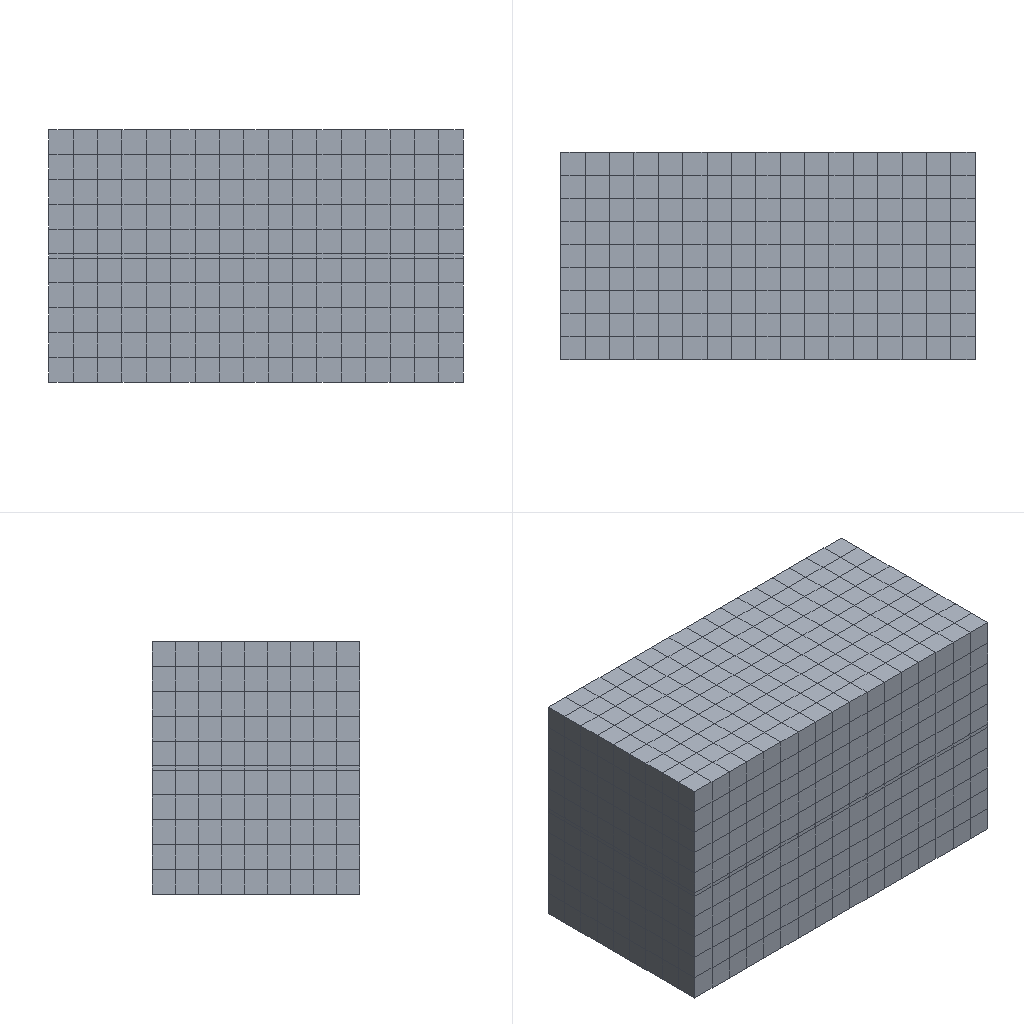Simulation study | ansys workbench
Ansys APDL input file, long lists of numbers shortened:
/batch
/config,noeldb,1     ! force off writing results to database
*get,_wallstrt,active,,time,wall
! ANSYS input file written by Workbench version 2022 R2
! File used for geometry attach:
/title,wbnew--___ (A5)
! ****** Begin Custom Load Command Snippet ******
/COM, ACT Extensions:
/COM,     LSDYNA, 2022.2
/COM,/COM,     ANSYSMotion, 2022.2
/COM,
! ****** End   Custom Load Command Snippet ******
*DIM,_wb_ProjectScratch_dir,string,248
_wb_ProjectScratch_dir(1) = ''
*DIM,_wb_SolverFiles_dir,string,248
_wb_SolverFiles_dir(1) = ''
*DIM,_wb_userfiles_dir,string,248
_wb_userfiles_dir(1) = ''
/com,--- Data in consistent NMM units. See Solving Units in the help system for more information.
/units,MPA
/nopr
/wb,file,start              !  signify a WB generated input file
/prep7
! Turn off shape checking because checks already performed inside WB mesher.
! See help system for more information.
SHPP,OFF,,NOWARN
/nolist
etcon,set             ! allow ANSYS to choose best KEYOP's for 180x elements, resets any applicable keyopt to MAPDL defaults
/com,*********** Nodes for the whole assembly ***********
nblock,3,,10062
(1i9,3e20.9e3)
     7945     4.411764706E+00     1.944444444E+00     3.000000000E+00
! (9147 more lines like these left out)
-1
/wb,elem,start            !  set before creation of elements
/com,*********** Elements for Body 1 "__" ***********
et,1,279
eblock,19,solid,,765
(19i9)
        1        1        1        1        0        0        0        0       20        0        1        1     1001      862      824      640     1080      861      853
! (1529 more lines like these left out)
-1
/com,*********** Elements for Body 2 "__" ***********
et,2,279
eblock,19,solid,,765
(19i9)
        2        2        2        2        0        0        0        0       20        0      766     3973     4793     4874     5041     4612     4872     4873     5045
! (1529 more lines like these left out)
-1
/com,*********** Elements for Body 3 "__" ***********
et,3,279
eblock,19,solid,,153
(19i9)
        3        3        3        3        0        0        0        0       20        0     1531     8072     8297     8269     8268     8073     8208     8235     8236
! (305 more lines like these left out)
-1
/wb,elem,end               !  done creating elements
/com,*********** Send User Defined Coordinate System(s) ***********
csys,0
toffst,273.15,  ! Temperature offset from absolute zero
/wb,mat,start              !  starting to send materials
/com,*********** Send Materials ***********
MP,DENS,1,3.2e-09,	! tonne mm^-3
MP,ALPX,1,3.5e-06,	! C^-1
MP,KXX,1,20,	! tonne mm s^-3 C^-1
MP,C,1,750000000,	! mm^2 s^-2 C^-1
MP,EX,1,300000,	! tonne s^-2 mm^-1
MP,NUXY,1,0.27,
Temperature = 'TEMP' ! Temperature
MP,DENS,2,4.51e-09,	! tonne mm^-3
MP,CTEX,2,9e-06,	! C^-1
MP,C,2,530000000,	! mm^2 s^-2 C^-1
MP,KXX,2,19,	! tonne mm s^-3 C^-1
MP,RSVX,2,0.0017,	! ohm mm
MP,EX,2,110000,	! tonne s^-2 mm^-1
MP,NUXY,2,0.34,
MP,MURX,2,1,
MP,DENS,3,9.8e-09,	! tonne mm^-3
MP,CTEX,3,1.9e-05,	! C^-1
MP,EX,3,75000,	! tonne s^-2 mm^-1
MP,NUXY,3,0.35,
MP,KXX,3,110,	! tonne mm s^-3 C^-1
MP,C,3,420000000,	! mm^2 s^-2 C^-1
/wb,mat,end                !  done sending materials
!************************* Model Summary ********************
!__,	SI3N4,	matid,	1
!__,	钛合金,	matid,	2
!__,	AG-CU-TI,	matid,	3
!************************* End Model Summary ********************
! get the diagonal of the bounding box. Needed later for other things
*get,_xmin,node,,mnloc,x
*get,_ymin,node,,mnloc,y
*get,_zmin,node,,mnloc,z
*get,_xmax,node,,mxloc,x
*get,_ymax,node,,mxloc,y
*get,_zmax,node,,mxloc,z
_ASMDIAG=(_xmax-_xmin)*(_xmax-_xmin)+(_ymax-_ymin)*(_ymax-_ymin)+(_zmax-_zmin)*(_zmax-_zmin)
_ASMDIAG=SQRT(_ASMDIAG)
/wb,contact,start          !  starting to send contact
/com,*********** Create Contact "接触区域" ***********
/com,            Real Constant Set For Above Contact Is 5 & 4
*set,tid,5
*set,cid,4
r,tid
r,cid
et,tid,170
et,cid,174
eblock,10,,,153
(15i9)
     3174        5        5        5        0      853      640     1080      861     3119     3120     3583     3574
! (152 more lines like these left out)
-1
eblock,10,,,153
(15i9)
     3327        4        4        4        0      853      640     1080      861     3119     3120     3583     3574
! (152 more lines like these left out)
-1
eblock,10,,,153
(15i9)
     3480        4        5        4        0     8236     8073     8208     8235     8716     8715     9008     9062
! (152 more lines like these left out)
-1
eblock,10,,,153
(15i9)
     3633        5        4        5        0     8236     8073     8208     8235     8716     8715     9008     9062
! (152 more lines like these left out)
-1
keyo,cid,8,2               ! auto create asymmetric contact (from Program Controlled setting)
keyo,cid,10,0              ! adjust contact stiffness each NR iteration (from Program Controlled setting)
keyo,cid,12,5              ! bonded always
keyo,cid,18,1              ! small sliding turned on by application
keyo,cid,2,0               ! augmented Lagrange (from Program Controlled setting)
keyo,cid,4,0               ! on Gauss point (from Program Controlled setting)
keyo,cid,9,1               ! ignore initial gaps/penetration
keyo,cid,7,0               ! No Prediction
rmod,tid,3,10.      ! FKN
rmod,tid,5,0.       ! ICONT
rmod,tid,6,0.       ! PINB
rmod,tid,10,0.      ! CNOF
rmod,tid,12,0.      ! FKT
rmod,tid,36,34      ! WB DSID
rmod,cid,3,10.      ! FKN
rmod,cid,5,0.       ! ICONT
rmod,cid,6,0.       ! PINB
rmod,cid,10,0.      ! CNOF
rmod,cid,12,0.      ! FKT
rmod,cid,36,34      ! WB DSID
*set,_maxkxx,1100000.
rmod,cid,14,_maxkxx/_ASMDIAG         ! TCC, Divide by Length since Traction Based
rmod,tid,14,_maxkxx/_ASMDIAG      ! TCC, Divide by Length since Traction Based
keyo,cid,1,2     ! Pure thermal contact
/com,*********** Create Contact "接触区域 2" ***********
/com,            Real Constant Set For Above Contact Is 7 & 6
*set,tid,7
*set,cid,6
r,tid
r,cid
et,tid,170
et,cid,174
eblock,10,,,153
(15i9)
     3786        7        7        7        0     4776     4613     4748     4775     7096     7095     7388     7442
! (152 more lines like these left out)
-1
eblock,10,,,153
(15i9)
     3939        6        6        6        0     4776     4613     4748     4775     7096     7095     7388     7442
! (152 more lines like these left out)
-1
eblock,10,,,153
(15i9)
     4092        6        7        6        0     8297     8072     8268     8269     8712     8711     9113     9114
! (152 more lines like these left out)
-1
eblock,10,,,153
(15i9)
     4245        7        6        7        0     8297     8072     8268     8269     8712     8711     9113     9114
! (152 more lines like these left out)
-1
keyo,cid,8,2               ! auto create asymmetric contact (from Program Controlled setting)
keyo,cid,10,0              ! adjust contact stiffness each NR iteration (from Program Controlled setting)
keyo,cid,12,5              ! bonded always
keyo,cid,18,1              ! small sliding turned on by application
keyo,cid,2,0               ! augmented Lagrange (from Program Controlled setting)
keyo,cid,4,0               ! on Gauss point (from Program Controlled setting)
keyo,cid,9,1               ! ignore initial gaps/penetration
keyo,cid,7,0               ! No Prediction
rmod,tid,3,10.      ! FKN
rmod,tid,5,0.       ! ICONT
rmod,tid,6,0.       ! PINB
rmod,tid,10,0.      ! CNOF
rmod,tid,12,0.      ! FKT
rmod,tid,36,37      ! WB DSID
rmod,cid,3,10.      ! FKN
rmod,cid,5,0.       ! ICONT
rmod,cid,6,0.       ! PINB
rmod,cid,10,0.      ! CNOF
rmod,cid,12,0.      ! FKT
rmod,cid,36,37      ! WB DSID
*set,_maxkxx,1100000.
rmod,cid,14,_maxkxx/_ASMDIAG         ! TCC, Divide by Length since Traction Based
rmod,tid,14,_maxkxx/_ASMDIAG      ! TCC, Divide by Length since Traction Based
keyo,cid,1,2     ! Pure thermal contact
nsel,all
esel,all
/wb,contact,end            !  done creating contacts
/golist
/wb,load,start             !  starting to send loads
/com,*********** Create "热流" ***********
et,8,152
eblock,10,,,17
(15i9)
     4398        8        8        8        0     8268     8236     8235     8269     9065     9062     9063     9113
! (16 more lines like these left out)
-1
esel,s,type,,8
keyop,8,8,1      ! include heat flux
esel,all
fcum,add                   ! add nodal forces up (needed in case have loads on the same edge,vertex)
nsel,all
nsel,all
fcum                       ! reset default on fcum command since done sending WB F loads
/com,*********** Create "______" ***********
et,9,152
eblock,10,,,826
(15i9)
     4415        9        9        9        0     1080     1001      862      861     3836     3585     3582     3583
! (825 more lines like these left out)
-1
esel,s,type,,9
keyop,9,8,2.
keyop,9,13,0
*DIM,_convvari62,TABLE,8,1,1,TEMP,
! Temperature values
_convvari62(1,0,1) = 1.
_convvari62(2,0,1) = 10.
_convvari62(3,0,1) = 100.
_convvari62(4,0,1) = 200.
_convvari62(5,0,1) = 300.
_convvari62(6,0,1) = 500.
_convvari62(7,0,1) = 700.
_convvari62(8,0,1) = 1000.
! Load values
_convvari62(1,1,1) = 1.24e-003
_convvari62(2,1,1) = 2.67e-003
_convvari62(3,1,1) = 5.76e-003
_convvari62(4,1,1) = 7.25e-003
_convvari62(5,1,1) = 8.3e-003
_convvari62(6,1,1) = 9.84e-003
_convvari62(7,1,1) = 1.101e-002
_convvari62(8,1,1) = 1.24e-002
esel,all
/com,*********** Create "ToAmbient" Radiation ***********
n,9149,_ASMDIAG*0.5*1,0.,0.
nsel,s,node,,9149
cm,_SPND64,node
nsel,all
et,10,152
keyop,10,5,1        !  Extra node
keyop,10,9,1        !  Use radiation with the form factor real constant
eblock,10,,,1490
(15i9)
     5241       10       10       10        0      819      821      865      820     3503     3507     3504     3502     9149
! (1489 more lines like these left out)
-1
esel,s,type,,10
mp,emis,10,0.3
r,10,1.,5.669e-011
stef,5.669e-011
esel,all
nsel,all
/com,***************** Define Uniform Initial temperature ***************
tunif,25.
/gst,on,on
fini
*get,_numnode,node,0,count
*get,_numelem,elem,0,count
*get, _MAXELEMNUM, elem, 0, NUM, MAX
*get, _MAXNODENUM, node, 0, NUM, MAX
*get, _MAXELEMTYPE, etyp, 0, NUM, MAX
*get, _MAXREALCONST, rcon, 0, NUM, MAX
/go
/wb,load,end               !  done creating loads
/com,--- Number of total nodes = %_numnode%
/com,--- Number of contact elements = 3557
/com,--- Number of spring elements = 0
/com,--- Number of bearing elements = 0
/com,--- Number of solid elements = 1683
/com,--- Number of condensed parts = 0
/com,--- Number of total elements = %_numelem%
*get,_wallbsol,active,,time,wall
/com,****************************************************************************
/com,*************************    SOLUTION       ********************************
/com,****************************************************************************
/solu
antype,4                   ! transient analysis
kbc,1                      ! stepped BC's
!eqsl,sparse               ! using sparse solver which is default so no eqsl command needed
cntr,print,1               ! print out contact info and also make no initial contact an error
rescontrol,,none                 ! Do not keep any restart files
dmpoption,emat,no             ! Don't combine emat file for DANSYS
dmpoption,esav,no             ! Don't combine esav file for DANSYS
thopt,full
nlhist,nsol,MAX_TEMP,temp,max
nlhist,nsol,MIN_TEMP,temp,min
/com,********* Initial Time Increment Check And Fourier Modulus *********
/com, Specified Initial Time Increment: 0.01
/com, Estimated Increment Needed, le*le/alpha, Body 1: 0.0405
/com, Estimated Increment Needed, le*le/alpha, Body 2: 0.04246
/com, Estimated Increment Needed, le*le/alpha, Body 3: 0.003825
/com,****************************************************
/com,******************* SOLVE FOR LS 1 OF 5 ****************
esel,s,type,,8
nsle
sf,all,hflux,200000.
nsel,all
esel,all
esel,s,type,,9
nsle
sf,all,conv,%_convvari62%,25.
nsel,all
esel,all
d,_SPND64,temp,25.
/nopr
/gopr
autots,on
nsub,100,1000,10
time,1.
timint,on                  ! Turn on time integration effects
outres,erase
outres,all,none
outres,nsol,all
outres,rsol,all
outres,eangl,all
outres,veng,all
outres,fflux,all
outres,cont,all
/nopr
esel,s,type,,9
esel,a,type,,10
cm,_elmisc,elem
esel,all
/gopr
outres,misc,all,_elmisc
cnvtol,heat,,.001,,1.e-003    ! Program Controlled. Set MINREF equivalent of 1e-6 Watts
! *********** WB SOLVE COMMAND ***********
! check interactive state
*get,ANSINTER_,active,,int
*if,ANSINTER_,ne,0,then
/eof
*endif
solve
/com *************** Write FE CONNECTORS *********
CEWRITE,file,ce,,INTE
/com,****************************************************
/com,*************** FINISHED SOLVE FOR LS 1 *************
/com,****************************************************
/com,******************* SOLVE FOR LS 2 OF 5 ****************
/nopr
/gopr
autots,on
nsub,100,1000,10
time,2.
timint,on                  ! Turn on time integration effects
outres,erase
outres,all,none
outres,nsol,all
outres,rsol,all
outres,eangl,all
outres,veng,all
outres,fflux,all
outres,cont,all
outres,misc,all,_elmisc
cnvtol,heat,,.001,,1.e-003    ! Program Controlled. Set MINREF equivalent of 1e-6 Watts
solve
/com,****************************************************
/com,*************** FINISHED SOLVE FOR LS 2 *************
/com,****************************************************
/com,******************* SOLVE FOR LS 3 OF 5 ****************
/nopr
/gopr
autots,on
nsub,100,1000,10
time,3.
timint,on                  ! Turn on time integration effects
outres,erase
outres,all,none
outres,nsol,all
outres,rsol,all
outres,eangl,all
outres,veng,all
outres,fflux,all
outres,cont,all
outres,misc,all,_elmisc
cnvtol,heat,,.001,,1.e-003    ! Program Controlled. Set MINREF equivalent of 1e-6 Watts
solve
/com,****************************************************
/com,*************** FINISHED SOLVE FOR LS 3 *************
/com,****************************************************
/com,******************* SOLVE FOR LS 4 OF 5 ****************
/nopr
/gopr
autots,on
nsub,100,1000,10
time,4.
timint,on                  ! Turn on time integration effects
outres,erase
outres,all,none
outres,nsol,all
outres,rsol,all
outres,eangl,all
outres,veng,all
outres,fflux,all
outres,cont,all
outres,misc,all,_elmisc
cnvtol,heat,,.001,,1.e-003    ! Program Controlled. Set MINREF equivalent of 1e-6 Watts
solve
/com,****************************************************
/com,*************** FINISHED SOLVE FOR LS 4 *************
/com,****************************************************
/com,******************* SOLVE FOR LS 5 OF 5 ****************
/nopr
/gopr
autots,on
nsub,100,1000,10
time,5.
timint,on                  ! Turn on time integration effects
outres,erase
outres,all,none
outres,nsol,all
outres,rsol,all
outres,eangl,all
outres,veng,all
outres,fflux,all
outres,cont,all
outres,misc,all,_elmisc
cnvtol,heat,,.001,,1.e-003    ! Program Controlled. Set MINREF equivalent of 1e-6 Watts
solve
/com,****************************************************
/com,*************** FINISHED SOLVE FOR LS 5 *************
*get,_wallasol,active,,time,wall
/post1
xmlo,ENCODING,ISO-8859-1
xmlo,parm
/xml,parm,xml
fini
/gopr
*get,_walldone,active,,time,wall
_preptime=(_wallbsol-_wallstrt)*3600
_solvtime=(_wallasol-_wallbsol)*3600
_posttime=(_walldone-_wallasol)*3600
_totaltim=(_walldone-_wallstrt)*3600
*get,_dlbratio,active,0,solu,dlbr
*get,_combtime,active,0,solu,comb
*get,_ssmode,active,0,solu,ssmm
*get,_ndofs,active,0,solu,ndof
/fclean				!clean distributed files
/com,--- Total number of nodes = %_numnode%
/com,--- Total number of elements = %_numelem%
/com,--- Element load balance ratio = %_dlbratio%
/com,--- Time to combine distributed files = %_combtime%
/com,--- Sparse memory mode = %_ssmode%
/com,--- Number of DOF = %_ndofs%
/wb,file,end               ! done with WB generated input